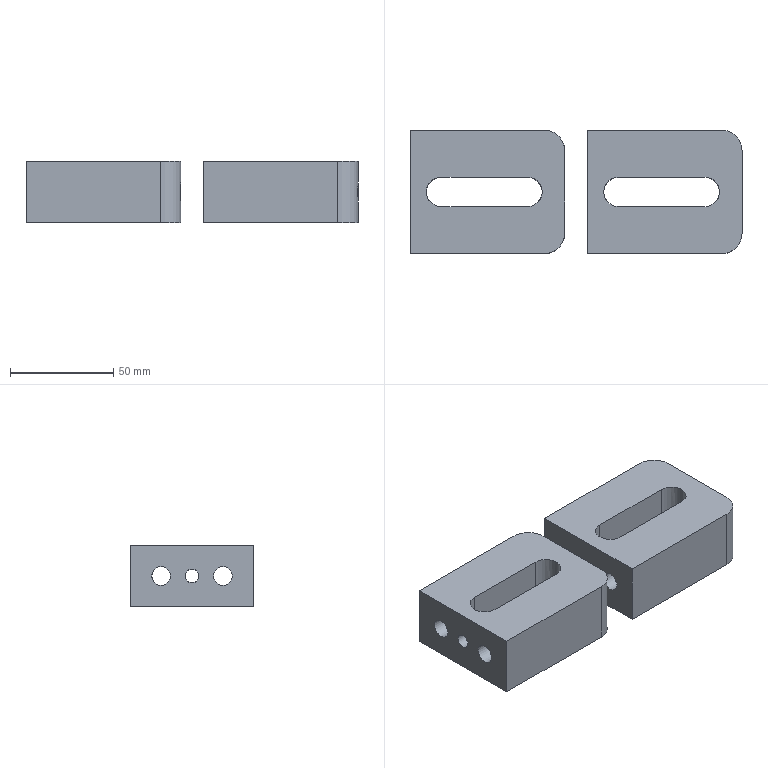Part | 2 solids | 62 faces | box 161 x 60 x 30 mm | volume 181737 mm3 | cylinder 32 | plane 22 | cone 8 | commonest cylinder face diameters 3.3 x8 6.6 x4 9 x4 14.2 x4 15 x4 20 x4